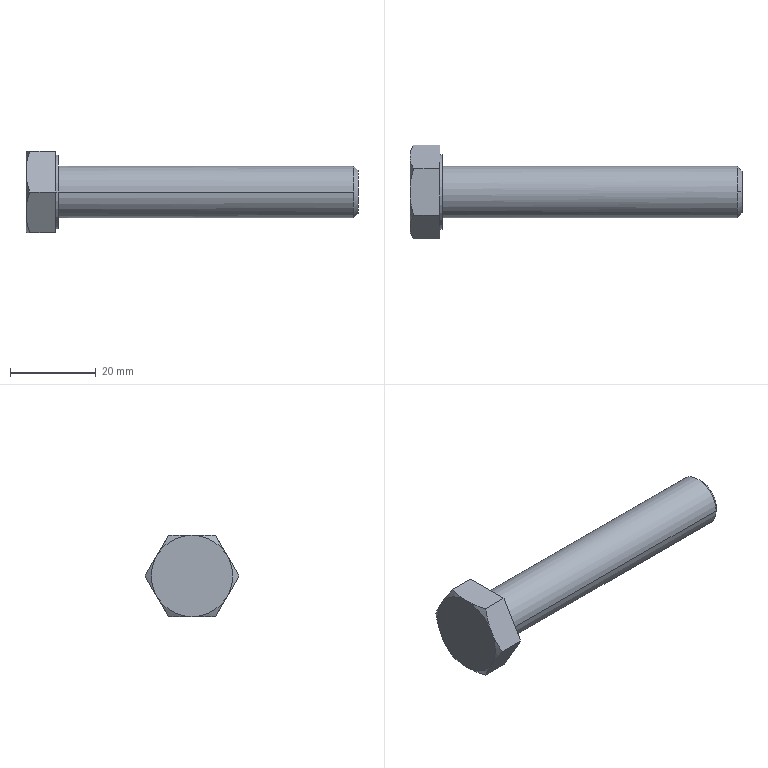Part | STEP file | DIN 931-1 - M12 x 70 | 1 solid | 22 faces | box 77.5 x 21.939 x 19 mm | volume 10189 mm3 | plane 10 | cone 8 | cylinder 4 | commonest cylinder face diameters 12 x2 17.4 x2